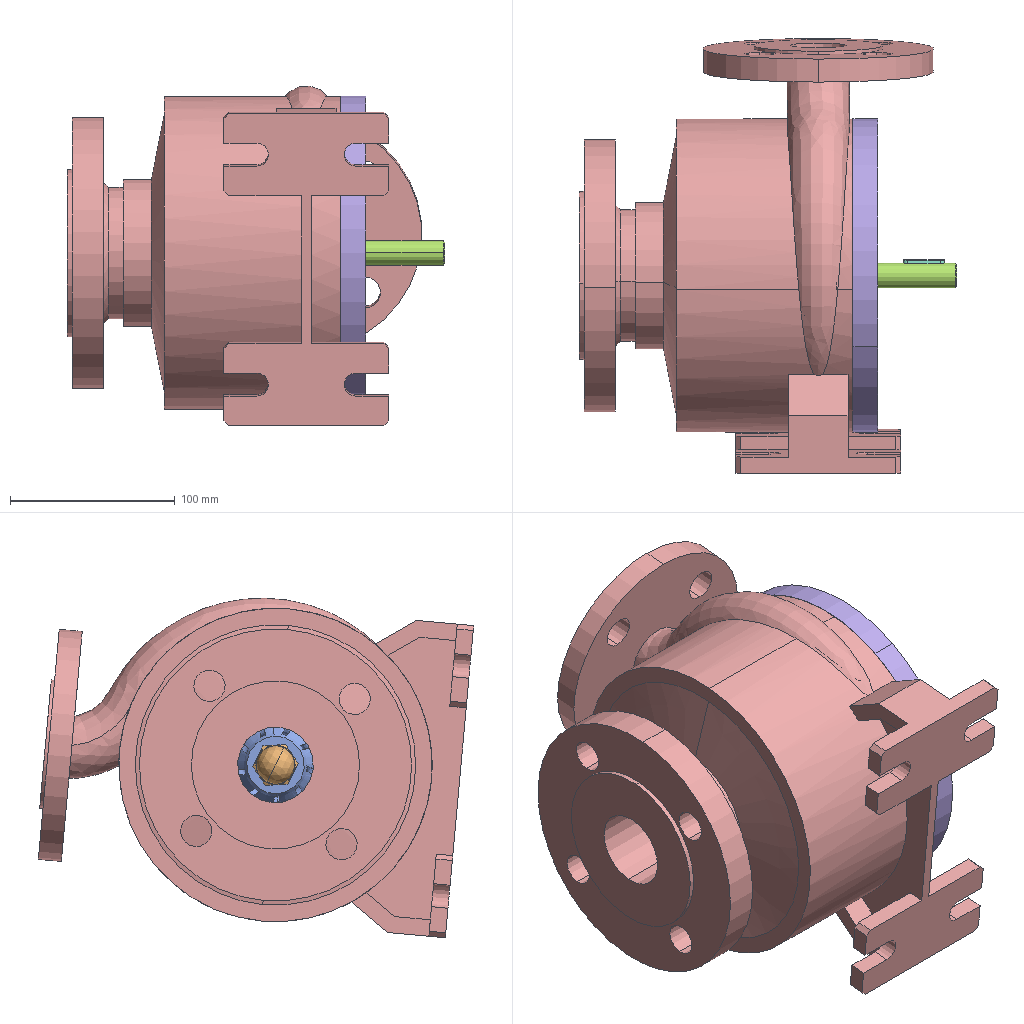Assembly | SolidWorks | 12 different items | 14 placed | box 229 x 264 x 206 mm
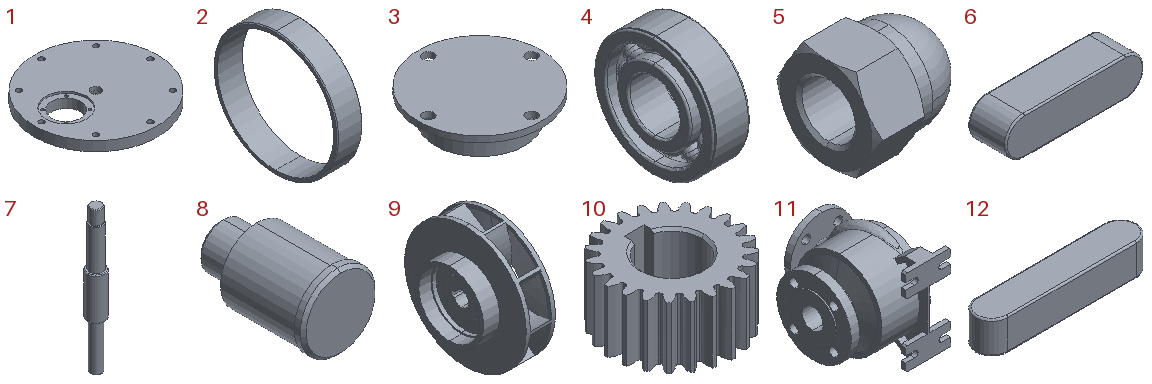Parts list (item | quantity | size | volume | features):
1 | x1 | 190 x 190 x 17 mm | 412970 mm3 | features ICE 4, Cut 2, Extrusion 1, HoleWzd 1
2 | x1 | 15 x 75 x 75 mm | 8483 mm3 | features Chamfer 1, Extrusion 1
3 | x1 | 62 x 62 x 15 mm | 19198 mm3 | features ICE 2, Cut 1, Extrusion 1
4 | x2 | 11 x 35 x 35 mm | 6458 mm3 | features Revolution 5, CirPattern 2, RevCut 2, RefAxis 1
5 | x1 | 28 x 27.713 x 24 mm | 7401 mm3 | features RevCut 5, Extrusion 1, Fillet 1, LPattern 1, Revolution 1
6 | x1 | 22 x 6 x 6 mm | 744.291 mm3 | features Extrusion 1, Fillet 1
7 | x1 | 24 x 24 x 199 mm | 54258 mm3 | features ICE 8, Chamfer 5, MoveFace 2, Cut 1, Revolution 1
8 | x1 | 25 x 40 x 25 mm | 14197 mm3 | features ICE 3, Chamfer 1, Extrusion 1
9 | x1 | 80 x 150 x 150 mm | 302851 mm3 | features ICE 3, CirPattern 1, Fillet 1, Revolution 1
10 | x2 | 49.96 x 49.854 x 25 mm | 28765 mm3 | features ICE 3, Chamfer 1, CirPattern 1, Extrusion 1, RefAxis 1
11 | x1 | 215 x 252 x 195.497 mm | 2163727 mm3 | features ICE 13, Fillet 3, Chamfer 2, Cut 2, MirrorPattern 2, Revolution 2, Blend 1, BlendCut 1, CirPattern 1, Helix 1, HoleWzd 1, MoveCopyBody 1, MoveFace 1, RevCut 1, Split 1
12 | x1 | 25 x 5 x 5 mm | 596.69 mm3 | features Extrusion 1, Fillet 1
Mates (type | each side: item.copy, entity, surface, feature):
Coincident | 11.1 axis | 2.1 axis
Coincident | 11.1 axis | 9.1 axis
Coincident | 9.1 face plane Revolve1 | 2.1 face plane Boss-Extrude1
Coincident | 11.1 face plane Revolve1 | 2.1 face plane Boss-Extrude1
Coincident | 7.1 face plane Cut-Extrude1 | 6.1 face plane Extrude1
Concentric | 7.1 face cylinder Cut-Extrude1 | 6.1 face cylinder Extrude1 | 2 times
Coincident | 7.1 face plane Revolve1 | 5.1 face plane Undercut
Concentric | 7.1 face cylinder Revolve1 | 5.1 face cylinder TapDrill
Parallel | 9.1 face plane Cut-Extrude1 | 6.1 face plane Extrude1
Concentric | 11.1 face cylinder CirPattern1 | 1.1 face cylinder Cut-Extrude5
Coincident | 1.1 face plane Cut-Extrude4 | 3.1 face plane Boss-Extrude1
Concentric | 1.1 face cylinder Cut-Extrude3 | 3.1 face cylinder Boss-Extrude1
Coincident | 11.1 face plane Revolve1 | 1.1 face plane Boss-Extrude1
Concentric | 11.1 face cylinder Revolve1 | 1.1 face cylinder Boss-Extrude1
Concentric | 1.1 face cylinder M5 Tapped Hole1 | 3.1 face cylinder Cut-Extrude2
Concentric | 11.1 face cylinder Cut-Extrude3 | 8.1 face cylinder Boss-Extrude2
Coincident | 11.1 face plane Cut-Extrude3 | 8.1 face plane Boss-Extrude1
Concentric | 11.1 face cylinder Cut-Extrude2 | 7.1 face cylinder Revolve1
Coincident | 7.1 face plane Boss-Extrude1 | 1.1 face plane Boss-Extrude2
Concentric | 7.1 face cylinder Revolve1 | 10.1 face cylinder Cut-Extrude2
Coincident | 7.1 face plane Boss-Extrude1 | 10.1 face plane Boss-Extrude1
Parallel | 7.1 face plane Cut-Extrude4 | 10.1 face plane Cut-Extrude3
Concentric | 8.1 face cylinder Boss-Extrude2 | 10.2 face cylinder Cut-Extrude2
Coincident | 10.1 face plane Boss-Extrude1 | 10.2 face plane Boss-Extrude1
Concentric | 8.1 face cylinder Boss-Extrude3 | 4.1 face cylinder Revolve1
Coincident | 3.1 face plane Cut-Extrude1 | 4.1 face plane Revolve1
Coincident | 7.1 edge | 4.2 face plane Revolve1
Concentric | 7.1 face cylinder Cut-Extrude7 | 12.1 face cylinder Base-Extrude
Coincident | 7.1 face plane Cut-Extrude7 | 12.1 face plane Base-Extrude | 2 times